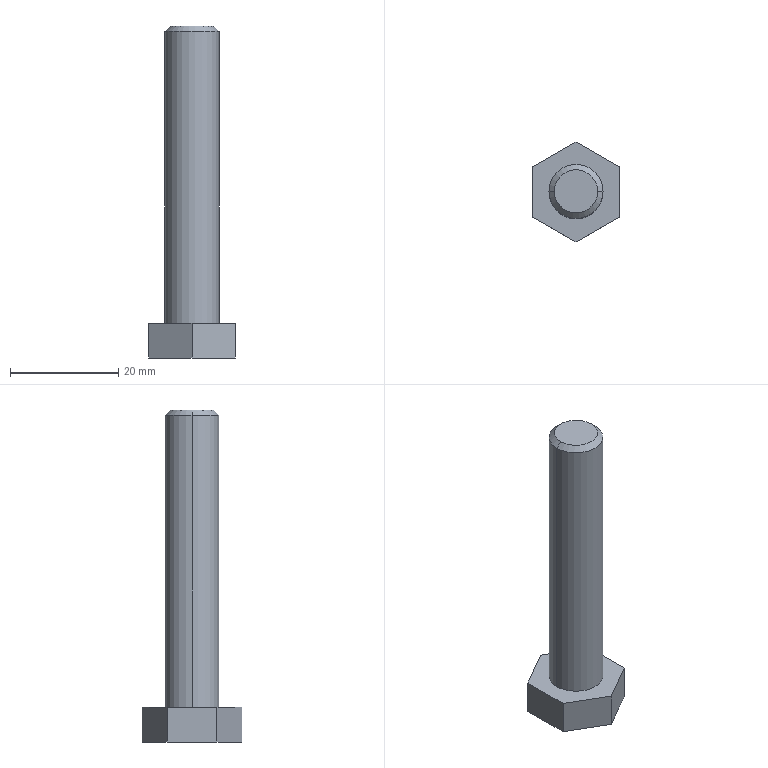Part | SolidWorks | features Chamfer 1, Extrusion 1, ICE 1, RefAxis 1 | 1 solid | 13 faces | box 16 x 18.475 x 61.4 mm | volume 5724 mm3 | plane 9 | cone 2 | cylinder 2 | commonest cylinder face diameters 10 x2
STEP:
#1=CARTESIAN_POINT('',(4.,0.,61.4));
#2=VERTEX_POINT('',#1);
#3=CARTESIAN_POINT('',(-4.,0.,61.4));
#4=VERTEX_POINT('',#3);
#5=CARTESIAN_POINT('',(0.,0.,61.4));
#6=DIRECTION('',(0.,0.,1.));
#7=DIRECTION('',(1.,0.,0.));
#8=AXIS2_PLACEMENT_3D('',#5,#6,#7);
#9=CIRCLE('',#8,4.);
#10=EDGE_CURVE('',#2,#4,#9,.T.);
#11=ORIENTED_EDGE('',*,*,#10,.F.);
#12=CARTESIAN_POINT('',(5.,0.,60.4));
#13=VERTEX_POINT('',#12);
#14=CARTESIAN_POINT('',(4.,0.,61.4));
#15=DIRECTION('',(0.7071,0.,-0.7071));
#16=VECTOR('',#15,1000.);
#17=LINE('',#14,#16);
#18=EDGE_CURVE('',#2,#13,#17,.T.);
#19=ORIENTED_EDGE('',*,*,#18,.T.);
#20=CARTESIAN_POINT('',(-5.,0.,60.4));
#21=VERTEX_POINT('',#20);
#22=CARTESIAN_POINT('',(0.,0.,60.4));
#23=DIRECTION('',(0.,0.,-1.));
#24=DIRECTION('',(1.,0.,0.));
#25=AXIS2_PLACEMENT_3D('',#22,#23,#24);
#26=CIRCLE('',#25,5.);
#27=EDGE_CURVE('',#21,#13,#26,.T.);
#28=ORIENTED_EDGE('',*,*,#27,.F.);
#29=CARTESIAN_POINT('',(-4.,0.,61.4));
#30=DIRECTION('',(-0.7071,0.,-0.7071));
#31=VECTOR('',#30,1000.);
#32=LINE('',#29,#31);
#33=EDGE_CURVE('',#4,#21,#32,.T.);
#34=ORIENTED_EDGE('',*,*,#33,.F.);
#35=EDGE_LOOP('',(#11,#19,#28,#34));
#36=FACE_OUTER_BOUND('',#35,.T.);
#37=CARTESIAN_POINT('',(0.,0.,61.4));
#38=DIRECTION('',(0.,0.,-1.));
#39=DIRECTION('',(-1.,0.,0.));
#40=AXIS2_PLACEMENT_3D('',#37,#38,#39);
#41=CONICAL_SURFACE('',#40,4.,0.7854);
#42=ADVANCED_FACE('',(#36),#41,.T.);
#43=ORIENTED_EDGE('',*,*,#27,.T.);
#44=CARTESIAN_POINT('',(5.,0.,6.4));
#45=VERTEX_POINT('',#44);
#46=CARTESIAN_POINT('',(5.,0.,61.4));
#47=DIRECTION('',(0.,0.,-1.));
#48=VECTOR('',#47,1000.);
#49=LINE('',#46,#48);
#50=EDGE_CURVE('',#13,#45,#49,.T.);
#51=ORIENTED_EDGE('',*,*,#50,.T.);
#52=CARTESIAN_POINT('',(-5.,0.,6.4));
#53=VERTEX_POINT('',#52);
#54=CARTESIAN_POINT('',(0.,0.,6.4));
#55=DIRECTION('',(0.,0.,1.));
#56=DIRECTION('',(1.,0.,0.));
#57=AXIS2_PLACEMENT_3D('',#54,#55,#56);
#58=CIRCLE('',#57,5.);
#59=EDGE_CURVE('',#45,#53,#58,.T.);
#60=ORIENTED_EDGE('',*,*,#59,.T.);
#61=CARTESIAN_POINT('',(-5.,0.,61.4));
#62=DIRECTION('',(0.,0.,-1.));
#63=VECTOR('',#62,1000.);
#64=LINE('',#61,#63);
#65=EDGE_CURVE('',#21,#53,#64,.T.);
#66=ORIENTED_EDGE('',*,*,#65,.F.);
#67=EDGE_LOOP('',(#43,#51,#60,#66));
#68=FACE_OUTER_BOUND('',#67,.T.);
#69=CARTESIAN_POINT('',(0.,0.,61.4));
#70=DIRECTION('',(0.,0.,-1.));
#71=DIRECTION('',(-1.,0.,0.));
#72=AXIS2_PLACEMENT_3D('',#69,#70,#71);
#73=CYLINDRICAL_SURFACE('',#72,5.);
#74=ADVANCED_FACE('',(#68),#73,.T.);
#75=CARTESIAN_POINT('',(8.,-4.619,6.4));
#76=VERTEX_POINT('',#75);
#77=CARTESIAN_POINT('',(8.,4.619,6.4));
#78=VERTEX_POINT('',#77);
#79=CARTESIAN_POINT('',(8.,-4.619,6.4));
#80=DIRECTION('',(0.,1.,0.));
#81=VECTOR('',#80,1000.);
#82=LINE('',#79,#81);
#83=EDGE_CURVE('',#76,#78,#82,.T.);
#84=ORIENTED_EDGE('',*,*,#83,.T.);
#85=CARTESIAN_POINT('',(0.,9.238,6.4));
#86=VERTEX_POINT('',#85);
#87=CARTESIAN_POINT('',(8.,4.619,6.4));
#88=DIRECTION('',(-0.866,0.5,0.));
#89=VECTOR('',#88,1000.);
#90=LINE('',#87,#89);
#91=EDGE_CURVE('',#78,#86,#90,.T.);
#92=ORIENTED_EDGE('',*,*,#91,.T.);
#93=CARTESIAN_POINT('',(-8.,4.619,6.4));
#94=VERTEX_POINT('',#93);
#95=CARTESIAN_POINT('',(0.,9.238,6.4));
#96=DIRECTION('',(-0.866,-0.5,0.));
#97=VECTOR('',#96,1000.);
#98=LINE('',#95,#97);
#99=EDGE_CURVE('',#86,#94,#98,.T.);
#100=ORIENTED_EDGE('',*,*,#99,.T.);
#101=CARTESIAN_POINT('',(-8.,-4.619,6.4));
#102=VERTEX_POINT('',#101);
#103=CARTESIAN_POINT('',(-8.,4.619,6.4));
#104=DIRECTION('',(0.,-1.,0.));
#105=VECTOR('',#104,1000.);
#106=LINE('',#103,#105);
#107=EDGE_CURVE('',#94,#102,#106,.T.);
#108=ORIENTED_EDGE('',*,*,#107,.T.);
#109=CARTESIAN_POINT('',(0.,-9.238,6.4));
#110=VERTEX_POINT('',#109);
#111=CARTESIAN_POINT('',(-8.,-4.619,6.4));
#112=DIRECTION('',(0.866,-0.5,0.));
#113=VECTOR('',#112,1000.);
#114=LINE('',#111,#113);
#115=EDGE_CURVE('',#102,#110,#114,.T.);
#116=ORIENTED_EDGE('',*,*,#115,.T.);
#117=CARTESIAN_POINT('',(0.,-9.238,6.4));
#118=DIRECTION('',(0.866,0.5,0.));
#119=VECTOR('',#118,1000.);
#120=LINE('',#117,#119);
#121=EDGE_CURVE('',#110,#76,#120,.T.);
#122=ORIENTED_EDGE('',*,*,#121,.T.);
#123=EDGE_LOOP('',(#84,#92,#100,#108,#116,#122));
#124=FACE_OUTER_BOUND('',#123,.T.);
#125=CARTESIAN_POINT('',(0.,0.,6.4));
#126=DIRECTION('',(0.,0.,1.));
#127=DIRECTION('',(1.,0.,0.));
#128=AXIS2_PLACEMENT_3D('',#125,#126,#127);
#129=CIRCLE('',#128,5.);
#130=EDGE_CURVE('',#53,#45,#129,.T.);
#131=ORIENTED_EDGE('',*,*,#130,.F.);
#132=ORIENTED_EDGE('',*,*,#59,.F.);
#133=EDGE_LOOP('',(#131,#132));
#134=FACE_BOUND('',#133,.T.);
#135=CARTESIAN_POINT('',(0.,0.,6.4));
#136=DIRECTION('',(0.,0.,1.));
#137=DIRECTION('',(1.,0.,0.));
#138=AXIS2_PLACEMENT_3D('',#135,#136,#137);
#139=PLANE('',#138);
#140=ADVANCED_FACE('',(#124,#134),#139,.T.);
#141=CARTESIAN_POINT('',(8.,-4.619,0.));
#142=VERTEX_POINT('',#141);
#143=CARTESIAN_POINT('',(8.,4.619,0.));
#144=VERTEX_POINT('',#143);
#145=CARTESIAN_POINT('',(8.,-4.619,0.));
#146=DIRECTION('',(0.,1.,0.));
#147=VECTOR('',#146,1000.);
#148=LINE('',#145,#147);
#149=EDGE_CURVE('',#142,#144,#148,.T.);
#150=ORIENTED_EDGE('',*,*,#149,.T.);
#151=CARTESIAN_POINT('',(8.,4.619,6.4));
#152=DIRECTION('',(0.,0.,-1.));
#153=VECTOR('',#152,1000.);
#154=LINE('',#151,#153);
#155=EDGE_CURVE('',#78,#144,#154,.T.);
#156=ORIENTED_EDGE('',*,*,#155,.F.);
#157=ORIENTED_EDGE('',*,*,#83,.F.);
#158=CARTESIAN_POINT('',(8.,-4.619,6.4));
#159=DIRECTION('',(0.,0.,-1.));
#160=VECTOR('',#159,1000.);
#161=LINE('',#158,#160);
#162=EDGE_CURVE('',#76,#142,#161,.T.);
#163=ORIENTED_EDGE('',*,*,#162,.T.);
#164=EDGE_LOOP('',(#150,#156,#157,#163));
#165=FACE_OUTER_BOUND('',#164,.T.);
#166=CARTESIAN_POINT('',(8.,-4.619,6.4));
#167=DIRECTION('',(-1.,0.,0.));
#168=DIRECTION('',(0.,-1.,0.));
#169=AXIS2_PLACEMENT_3D('',#166,#167,#168);
#170=PLANE('',#169);
#171=ADVANCED_FACE('',(#165),#170,.F.);
#172=CARTESIAN_POINT('',(0.,9.238,0.));
#173=VERTEX_POINT('',#172);
#174=CARTESIAN_POINT('',(8.,4.619,0.));
#175=DIRECTION('',(-0.866,0.5,0.));
#176=VECTOR('',#175,1000.);
#177=LINE('',#174,#176);
#178=EDGE_CURVE('',#144,#173,#177,.T.);
#179=ORIENTED_EDGE('',*,*,#178,.T.);
#180=CARTESIAN_POINT('',(0.,9.238,6.4));
#181=DIRECTION('',(0.,0.,-1.));
#182=VECTOR('',#181,1000.);
#183=LINE('',#180,#182);
#184=EDGE_CURVE('',#86,#173,#183,.T.);
#185=ORIENTED_EDGE('',*,*,#184,.F.);
#186=ORIENTED_EDGE('',*,*,#91,.F.);
#187=ORIENTED_EDGE('',*,*,#155,.T.);
#188=EDGE_LOOP('',(#179,#185,#186,#187));
#189=FACE_OUTER_BOUND('',#188,.T.);
#190=CARTESIAN_POINT('',(8.,4.619,6.4));
#191=DIRECTION('',(-0.5,-0.866,0.));
#192=DIRECTION('',(0.866,-0.5,0.));
#193=AXIS2_PLACEMENT_3D('',#190,#191,#192);
#194=PLANE('',#193);
#195=ADVANCED_FACE('',(#189),#194,.F.);
#196=CARTESIAN_POINT('',(-8.,4.619,0.));
#197=VERTEX_POINT('',#196);
#198=CARTESIAN_POINT('',(0.,9.238,0.));
#199=DIRECTION('',(-0.866,-0.5,0.));
#200=VECTOR('',#199,1000.);
#201=LINE('',#198,#200);
#202=EDGE_CURVE('',#173,#197,#201,.T.);
#203=ORIENTED_EDGE('',*,*,#202,.T.);
#204=CARTESIAN_POINT('',(-8.,4.619,6.4));
#205=DIRECTION('',(0.,0.,-1.));
#206=VECTOR('',#205,1000.);
#207=LINE('',#204,#206);
#208=EDGE_CURVE('',#94,#197,#207,.T.);
#209=ORIENTED_EDGE('',*,*,#208,.F.);
#210=ORIENTED_EDGE('',*,*,#99,.F.);
#211=ORIENTED_EDGE('',*,*,#184,.T.);
#212=EDGE_LOOP('',(#203,#209,#210,#211));
#213=FACE_OUTER_BOUND('',#212,.T.);
#214=CARTESIAN_POINT('',(0.,9.238,6.4));
#215=DIRECTION('',(0.5,-0.866,0.));
#216=DIRECTION('',(0.866,0.5,0.));
#217=AXIS2_PLACEMENT_3D('',#214,#215,#216);
#218=PLANE('',#217);
#219=ADVANCED_FACE('',(#213),#218,.F.);
#220=CARTESIAN_POINT('',(-8.,-4.619,0.));
#221=VERTEX_POINT('',#220);
#222=CARTESIAN_POINT('',(-8.,4.619,0.));
#223=DIRECTION('',(0.,-1.,0.));
#224=VECTOR('',#223,1000.);
#225=LINE('',#222,#224);
#226=EDGE_CURVE('',#197,#221,#225,.T.);
#227=ORIENTED_EDGE('',*,*,#226,.T.);
#228=CARTESIAN_POINT('',(-8.,-4.619,6.4));
#229=DIRECTION('',(0.,0.,-1.));
#230=VECTOR('',#229,1000.);
#231=LINE('',#228,#230);
#232=EDGE_CURVE('',#102,#221,#231,.T.);
#233=ORIENTED_EDGE('',*,*,#232,.F.);
#234=ORIENTED_EDGE('',*,*,#107,.F.);
#235=ORIENTED_EDGE('',*,*,#208,.T.);
#236=EDGE_LOOP('',(#227,#233,#234,#235));
#237=FACE_OUTER_BOUND('',#236,.T.);
#238=CARTESIAN_POINT('',(-8.,4.619,6.4));
#239=DIRECTION('',(1.,0.,0.));
#240=DIRECTION('',(0.,1.,0.));
#241=AXIS2_PLACEMENT_3D('',#238,#239,#240);
#242=PLANE('',#241);
#243=ADVANCED_FACE('',(#237),#242,.F.);
#244=CARTESIAN_POINT('',(0.,-9.238,0.));
#245=VERTEX_POINT('',#244);
#246=CARTESIAN_POINT('',(-8.,-4.619,0.));
#247=DIRECTION('',(0.866,-0.5,0.));
#248=VECTOR('',#247,1000.);
#249=LINE('',#246,#248);
#250=EDGE_CURVE('',#221,#245,#249,.T.);
#251=ORIENTED_EDGE('',*,*,#250,.T.);
#252=CARTESIAN_POINT('',(0.,-9.238,6.4));
#253=DIRECTION('',(0.,0.,-1.));
#254=VECTOR('',#253,1000.);
#255=LINE('',#252,#254);
#256=EDGE_CURVE('',#110,#245,#255,.T.);
#257=ORIENTED_EDGE('',*,*,#256,.F.);
#258=ORIENTED_EDGE('',*,*,#115,.F.);
#259=ORIENTED_EDGE('',*,*,#232,.T.);
#260=EDGE_LOOP('',(#251,#257,#258,#259));
#261=FACE_OUTER_BOUND('',#260,.T.);
#262=CARTESIAN_POINT('',(-8.,-4.619,6.4));
#263=DIRECTION('',(0.5,0.866,0.));
#264=DIRECTION('',(-0.866,0.5,0.));
#265=AXIS2_PLACEMENT_3D('',#262,#263,#264);
#266=PLANE('',#265);
#267=ADVANCED_FACE('',(#261),#266,.F.);
#268=CARTESIAN_POINT('',(0.,-9.238,0.));
#269=DIRECTION('',(0.866,0.5,0.));
#270=VECTOR('',#269,1000.);
#271=LINE('',#268,#270);
#272=EDGE_CURVE('',#245,#142,#271,.T.);
#273=ORIENTED_EDGE('',*,*,#272,.T.);
#274=ORIENTED_EDGE('',*,*,#162,.F.);
#275=ORIENTED_EDGE('',*,*,#121,.F.);
#276=ORIENTED_EDGE('',*,*,#256,.T.);
#277=EDGE_LOOP('',(#273,#274,#275,#276));
#278=FACE_OUTER_BOUND('',#277,.T.);
#279=CARTESIAN_POINT('',(0.,-9.238,6.4));
#280=DIRECTION('',(-0.5,0.866,0.));
#281=DIRECTION('',(-0.866,-0.5,0.));
#282=AXIS2_PLACEMENT_3D('',#279,#280,#281);
#283=PLANE('',#282);
#284=ADVANCED_FACE('',(#278),#283,.F.);
#285=ORIENTED_EDGE('',*,*,#149,.F.);
#286=ORIENTED_EDGE('',*,*,#272,.F.);
#287=ORIENTED_EDGE('',*,*,#250,.F.);
#288=ORIENTED_EDGE('',*,*,#226,.F.);
#289=ORIENTED_EDGE('',*,*,#202,.F.);
#290=ORIENTED_EDGE('',*,*,#178,.F.);
#291=EDGE_LOOP('',(#285,#286,#287,#288,#289,#290));
#292=FACE_OUTER_BOUND('',#291,.T.);
#293=CARTESIAN_POINT('',(0.,0.,0.));
#294=DIRECTION('',(0.,0.,1.));
#295=DIRECTION('',(1.,0.,0.));
#296=AXIS2_PLACEMENT_3D('',#293,#294,#295);
#297=PLANE('',#296);
#298=ADVANCED_FACE('',(#292),#297,.F.);
#299=ORIENTED_EDGE('',*,*,#50,.F.);
#300=CARTESIAN_POINT('',(0.,0.,60.4));
#301=DIRECTION('',(0.,0.,-1.));
#302=DIRECTION('',(1.,0.,0.));
#303=AXIS2_PLACEMENT_3D('',#300,#301,#302);
#304=CIRCLE('',#303,5.);
#305=EDGE_CURVE('',#13,#21,#304,.T.);
#306=ORIENTED_EDGE('',*,*,#305,.T.);
#307=ORIENTED_EDGE('',*,*,#65,.T.);
#308=ORIENTED_EDGE('',*,*,#130,.T.);
#309=EDGE_LOOP('',(#299,#306,#307,#308));
#310=FACE_OUTER_BOUND('',#309,.T.);
#311=CARTESIAN_POINT('',(0.,0.,61.4));
#312=DIRECTION('',(0.,0.,-1.));
#313=DIRECTION('',(-1.,0.,0.));
#314=AXIS2_PLACEMENT_3D('',#311,#312,#313);
#315=CYLINDRICAL_SURFACE('',#314,5.);
#316=ADVANCED_FACE('',(#310),#315,.T.);
#317=CARTESIAN_POINT('',(0.,0.,61.4));
#318=DIRECTION('',(0.,0.,1.));
#319=DIRECTION('',(1.,0.,0.));
#320=AXIS2_PLACEMENT_3D('',#317,#318,#319);
#321=CIRCLE('',#320,4.);
#322=EDGE_CURVE('',#4,#2,#321,.T.);
#323=ORIENTED_EDGE('',*,*,#322,.T.);
#324=ORIENTED_EDGE('',*,*,#10,.T.);
#325=EDGE_LOOP('',(#323,#324));
#326=FACE_OUTER_BOUND('',#325,.T.);
#327=CARTESIAN_POINT('',(0.,0.,61.4));
#328=DIRECTION('',(0.,0.,1.));
#329=DIRECTION('',(1.,0.,0.));
#330=AXIS2_PLACEMENT_3D('',#327,#328,#329);
#331=PLANE('',#330);
#332=ADVANCED_FACE('',(#326),#331,.T.);
#333=ORIENTED_EDGE('',*,*,#18,.F.);
#334=ORIENTED_EDGE('',*,*,#322,.F.);
#335=ORIENTED_EDGE('',*,*,#33,.T.);
#336=ORIENTED_EDGE('',*,*,#305,.F.);
#337=EDGE_LOOP('',(#333,#334,#335,#336));
#338=FACE_OUTER_BOUND('',#337,.T.);
#339=CARTESIAN_POINT('',(0.,0.,61.4));
#340=DIRECTION('',(0.,0.,-1.));
#341=DIRECTION('',(-1.,0.,0.));
#342=AXIS2_PLACEMENT_3D('',#339,#340,#341);
#343=CONICAL_SURFACE('',#342,4.,0.7854);
#344=ADVANCED_FACE('',(#338),#343,.T.);
#345=CLOSED_SHELL('',(#42,#74,#140,#171,#195,#219,#243,#267,#284,#298,#316,#332,#344));
#346=MANIFOLD_SOLID_BREP('',#345);
#347=CARTESIAN_POINT('',(0.,0.,0.));
#348=DIRECTION('',(0.,0.,1.));
#349=DIRECTION('',(1.,0.,0.));
#350=AXIS2_PLACEMENT_3D('',#347,#348,#349);
#351=(LENGTH_UNIT()NAMED_UNIT(*)SI_UNIT(.MILLI.,.METRE.));
#352=UNCERTAINTY_MEASURE_WITH_UNIT(LENGTH_MEASURE(0.00001),#351,'','');
#353=(NAMED_UNIT(*)PLANE_ANGLE_UNIT()SI_UNIT($,.RADIAN.));
#354=(NAMED_UNIT(*)SI_UNIT($,.STERADIAN.)SOLID_ANGLE_UNIT());
#355=(GEOMETRIC_REPRESENTATION_CONTEXT(3)GLOBAL_UNCERTAINTY_ASSIGNED_CONTEXT((#352))GLOBAL_UNIT_ASSIGNED_CONTEXT((#351,#353,#354))REPRESENTATION_CONTEXT('',''));
#356=ADVANCED_BREP_SHAPE_REPRESENTATION('',(#346,#350),#355);